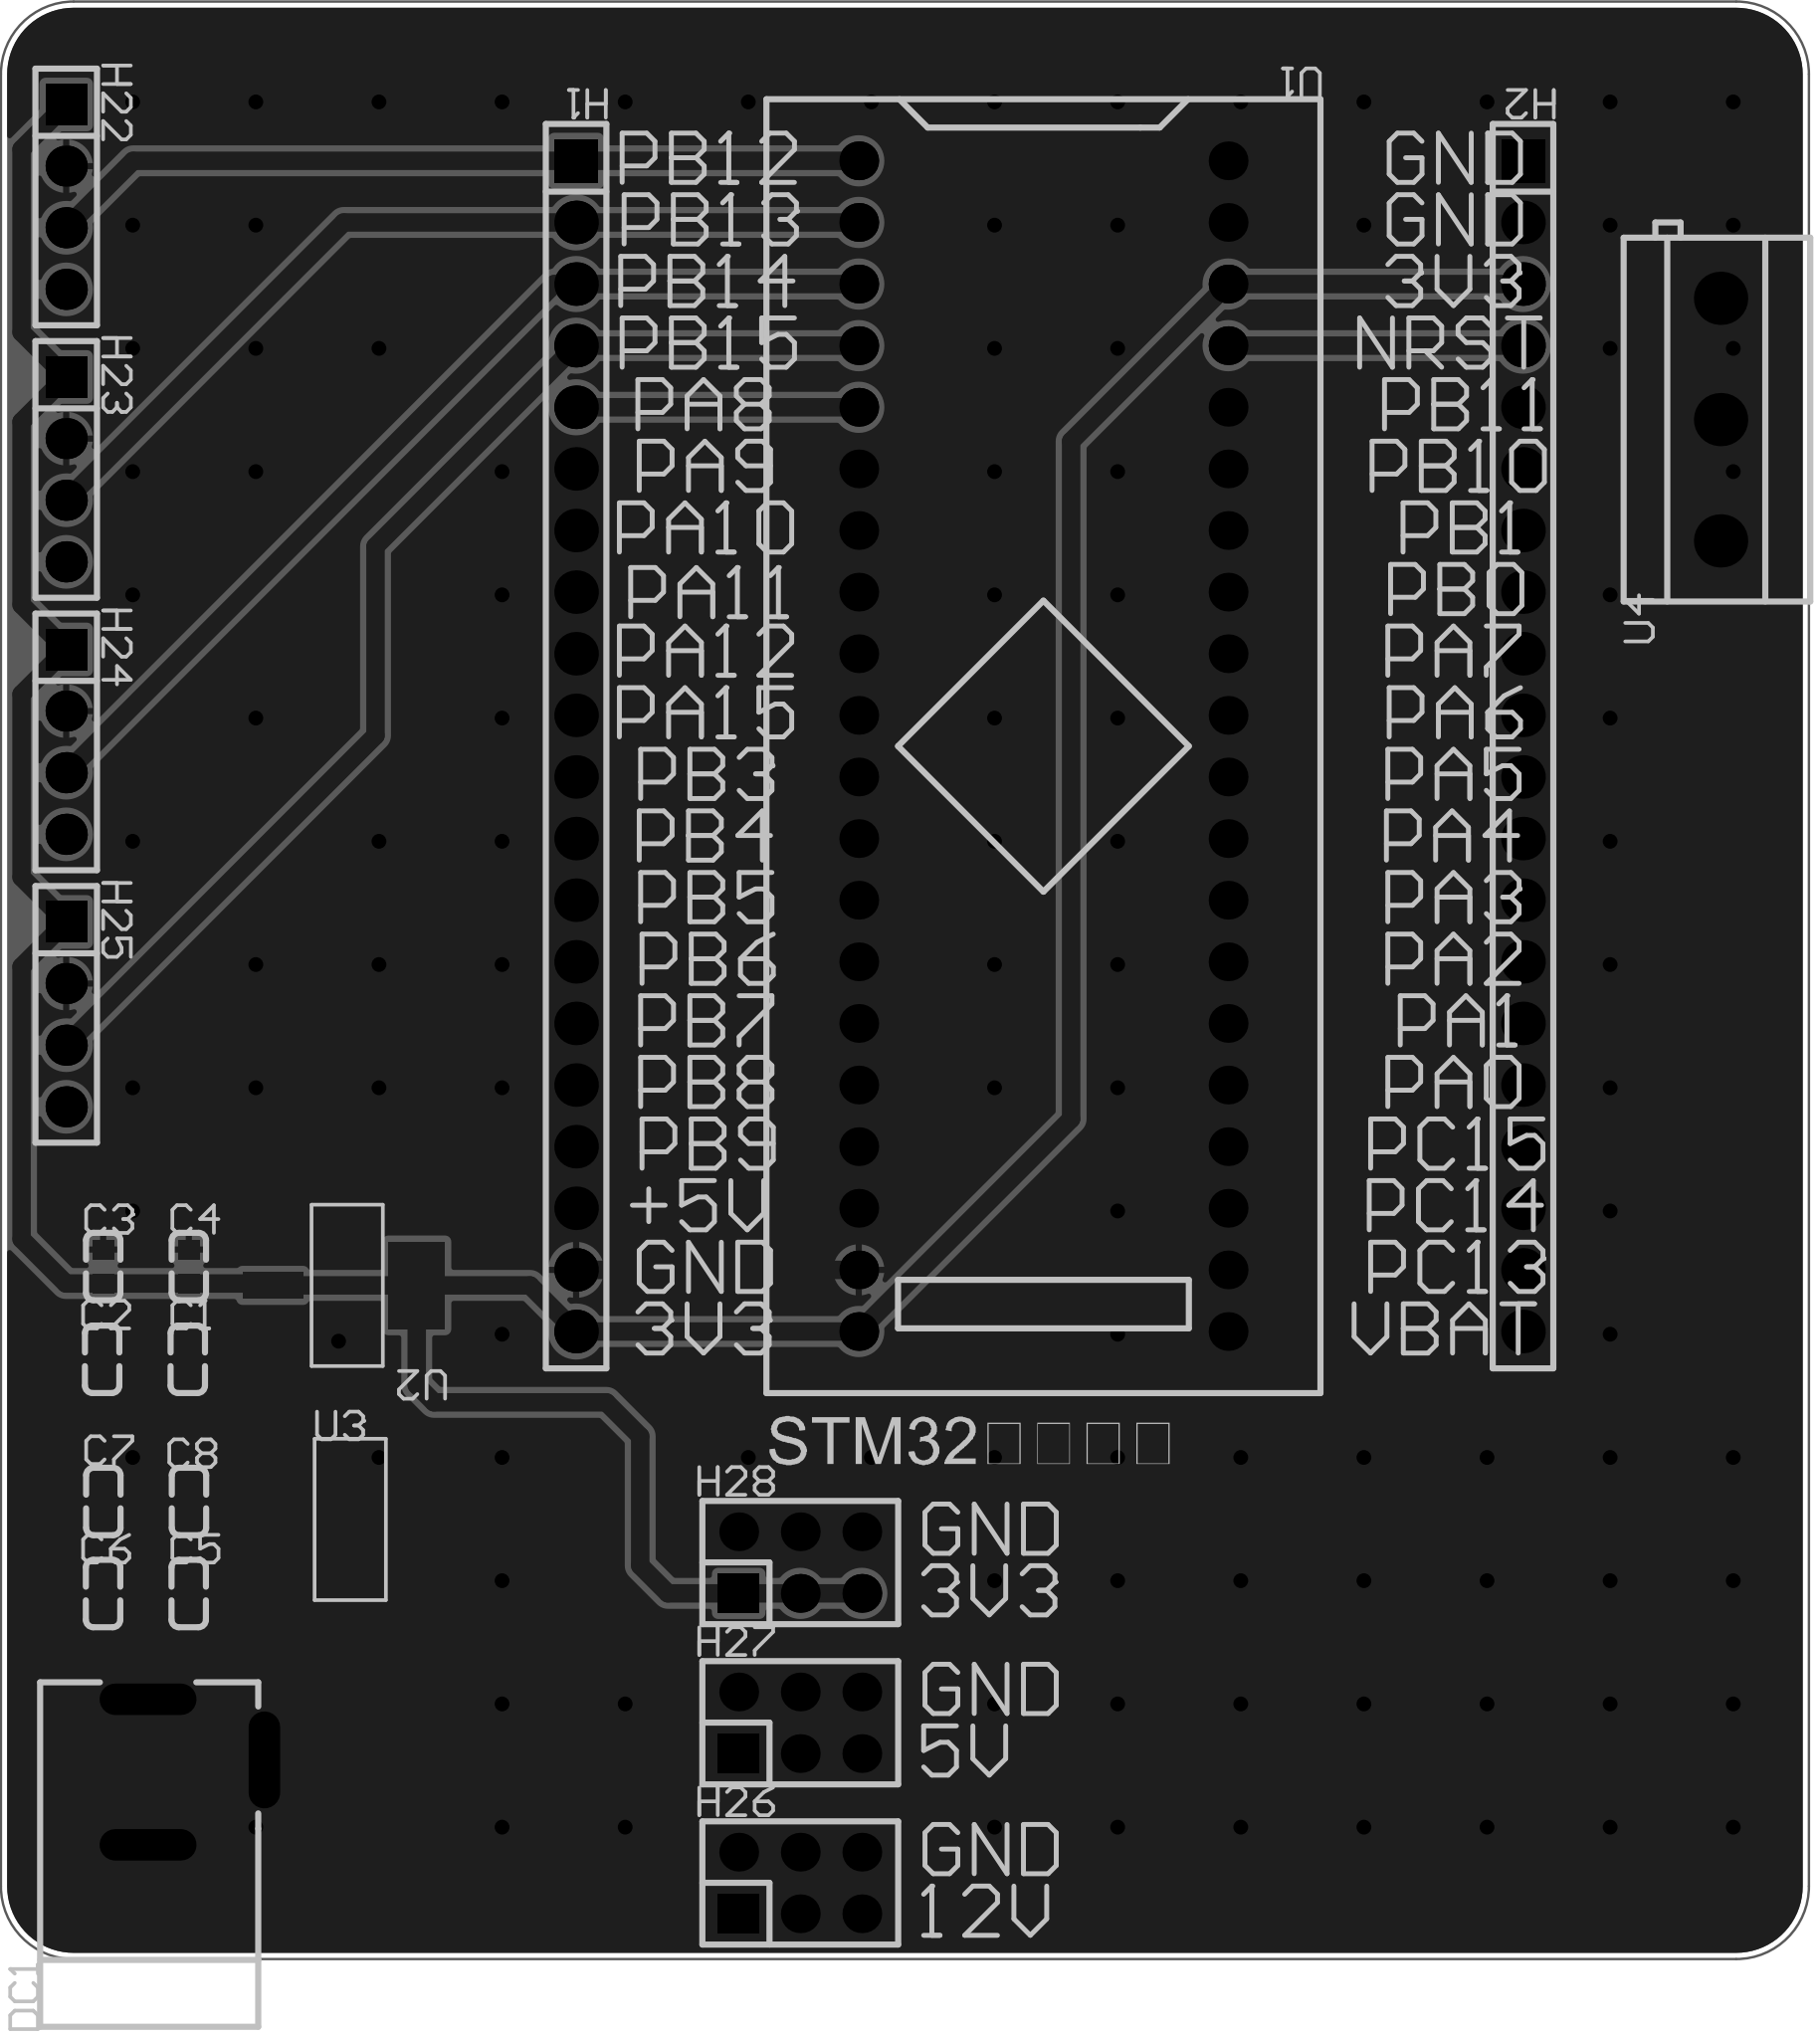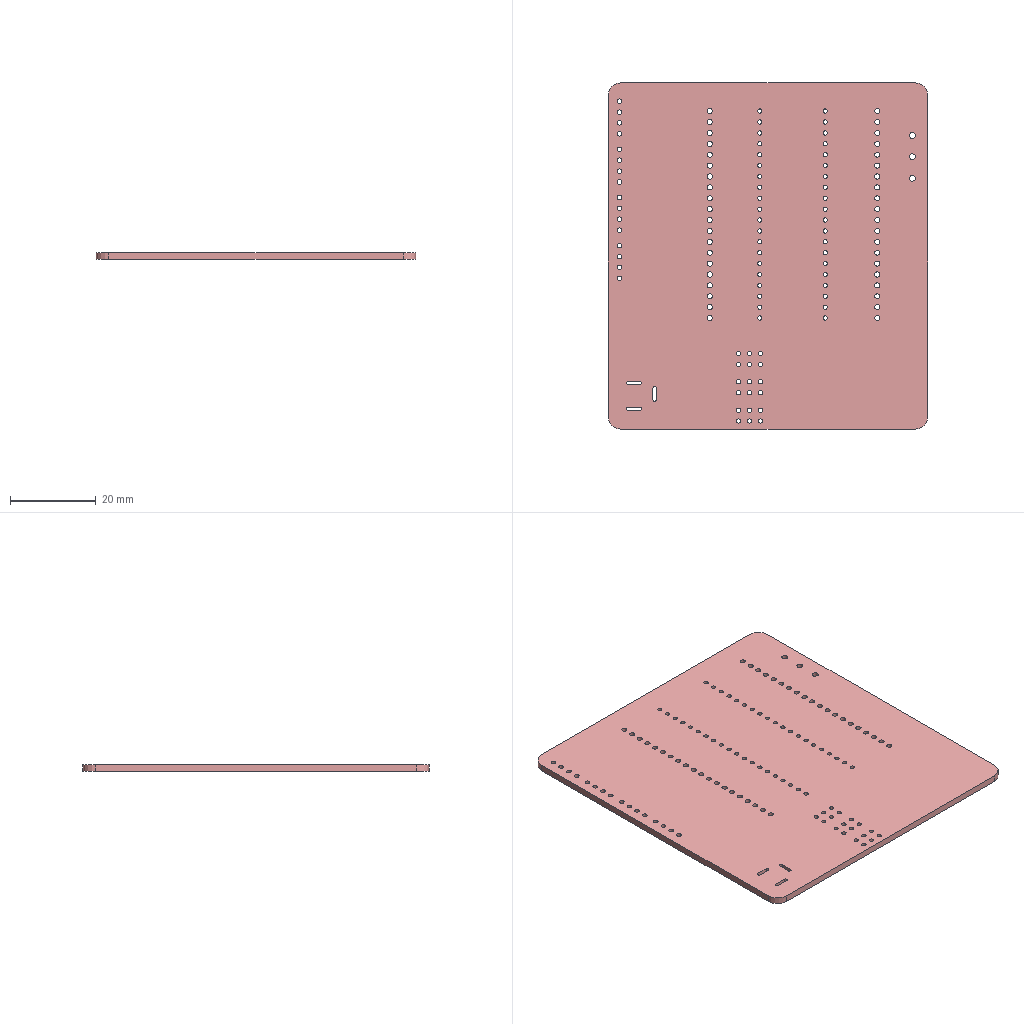Circuit board layout | Altium Designer | box 74.6 x 80.7 x 1.6 mm
Layer stack:
# Altium Designer layer stack of  (unit mm; dielectric type: 0 none, 1 core, 2 prepreg, 3 surface material)
index,name,kind,layer,copper_thickness_mm,dielectric_type,dielectric_thickness_mm,dielectric_material,dielectric_constant
0,Top Paste Mask Layer,other,,,,,,
1,Top Silkscreen Layer,other,,,,,,
2,Top Solder Mask Layer,dielectric,,,3,0.01,,3.3
3,Top Layer,copper,Top Layer,0.035,,,,
4,Dielectric1,dielectric,,,3,1.51,FR4,4.5
5,Bottom Layer,copper,Bottom Layer,0.035,,,,
6,Bottom Solder Mask Layer,dielectric,,,3,0.01,,3.3
7,Bottom Silkscreen Layer,other,,,,,,
8,Bottom Paste Mask Layer,other,,,,,,
# drill layer pairs: low layer,high layer
drill_pair,Top Layer,Bottom Layer
Part placement:
Designator,Comment,Layer,Footprint,Center-X(mm),Center-Y(mm),Rotation
U1,STM32F103C8T6-Card,TopLayer,CONN-TH_L53.3-W22.9_STM32F103C8T6-CARD,141.732,129.032,270
C1,100nF,TopLayer,C0603,106.427,103.756,90
C2,10uF,TopLayer,C0603,102.893,103.756,90
C3,100nF,TopLayer,C0603,102.936,107.581,270
C4,10uF,TopLayer,C0603,106.47,107.581,270
H1,,TopLayer,HDR-TH_20P-P2.54-V-F,122.449,129.032,270
H2,,TopLayer,HDR-TH_20P-P2.54-V-F,161.52,129.032,270
U2,AMS1117-3.3,TopLayer,SOT-223-3_L6.5-W3.4-P2.30-LS7.0-BR,112.904,106.804,180
C5,100nF,TopLayer,C0603,106.465,94.1,90
C6,10uF,TopLayer,C0603,102.931,94.1,90
C7,100nF,TopLayer,C0603,102.942,97.895,270
C8,10uF,TopLayer,C0603,106.476,97.895,270
DC1,,TopLayer,DC-2.0,107.188,86.741,270
H22,,TopLayer,HDR-TH_4P-P2.54-V-F,101.411,151.672,270
H23,,TopLayer,HDR-TH_4P-P2.54-V-F,101.411,140.44,270
H24,,TopLayer,HDR-TH_4P-P2.54-V-F,101.411,129.208,270
H25,,TopLayer,HDR-TH_4P-P2.54-V-F,101.411,117.975,270
H26,,TopLayer,HDR-TH_6P-P2.54-V-F-R2-C3-S2.54,131.699,82.169,0
H27,,TopLayer,HDR-TH_6P-P2.54-V-F-R2-C3-S2.54,131.699,88.773,0
H28,,TopLayer,HDR-TH_6P-P2.54-V-F-R2-C3-S2.54,131.699,95.377,0
U3,AMS1117-5.0,TopLayer,SOT-223-3_L6.5-W3.4-P2.30-LS7.0-BR,113.03,97.155,180
U4,KF301-5.0-3P,TopLayer,CONN-TH_3P-P5.00_KF301-5.0-3P,169.672,142.494,90
Pad and via stacks:
# Altium Designer via and pad stacks of  (unit mm). Each distinct definition once, with the count of objects using it.
# via: kind,start_layer,end_layer,hole_mm,diameter_mm,mode(0 simple;1 top-mid-bottom;2 full stack),diameter_per_layer,count,example_net
# pad: kind,layer,hole_mm,hole_type(0 round;1 square;2 slot),plating,top_size,top_shape(1 round;2 rect;3 octagon;9 rounded rect),mid_size,bottom_size,mode,footprint,size_per_layer,count,example
pad,Multi-Layer,1,0,plated,1.6x1.6,1,1.6x1.6,1.6x1.6,0,CONN-TH_L53.3-W22.9_STM32F103C8T6-CARD,,40,U1.1
pad,Multi-Layer,1.2,0,plated,1.8x1.8,2,1.8x1.8,1.8x1.8,0,HDR-TH_20P-P2.54-V-F,,2,H1.1
pad,Multi-Layer,1.2,0,plated,1.8x1.8,1,1.8x1.8,1.8x1.8,0,HDR-TH_20P-P2.54-V-F,,38,H1.2
pad,Multi-Layer,0.8001,2,plated,4x1.3,1,4x1.3,4x1.3,0,DC-2.0,,3,DC1.2
pad,Multi-Layer,1.1,0,plated,1.7x1.7,2,1.7x1.7,1.7x1.7,0,HDR-TH_4P-P2.54-V-F,,4,H22.1
pad,Multi-Layer,1.1,0,plated,1.7x1.7,1,1.7x1.7,1.7x1.7,0,HDR-TH_4P-P2.54-V-F,,12,H22.2
pad,Multi-Layer,1,0,plated,1.7x1.6,2,1.7x1.6,1.7x1.6,0,HDR-TH_6P-P2.54-V-F-R2-C3-S2.54,,3,H26.1
pad,Multi-Layer,1,0,plated,1.6x1.6,1,1.6x1.6,1.6x1.6,0,HDR-TH_6P-P2.54-V-F-R2-C3-S2.54,,15,H26.2
pad,Multi-Layer,1.4,0,plated,2.2x2.2,1,2.2x2.2,2.2x2.2,0,CONN-TH_3P-P5.00_KF301-5.0-3P,,3,U4.1
pad,Top Layer,0,0,plated,0.8x0.9,2,0.8x0.9,0.8x0.9,0,C0603,,16,C1.2
pad,Top Layer,0,0,plated,2.5x1.1,2,2.5x1.1,2.5x1.1,0,SOT-223-3_L6.5-W3.4-P2.30-LS7.0-BR,,6,U2.1
pad,Top Layer,0,0,plated,2.34x3.6,2,2.34x3.6,2.34x3.6,0,SOT-223-3_L6.5-W3.4-P2.30-LS7.0-BR,,2,U2.4
via,Top Layer,Bottom Layer,0.3048,0.61,0,,109,+5V
Copper pours:
name,layer,net,type(0 solid;1 hatched;2 none)
Bottom Layer-GND,Bottom Layer,GND,0
Top Layer-GND,Top Layer,GND,0